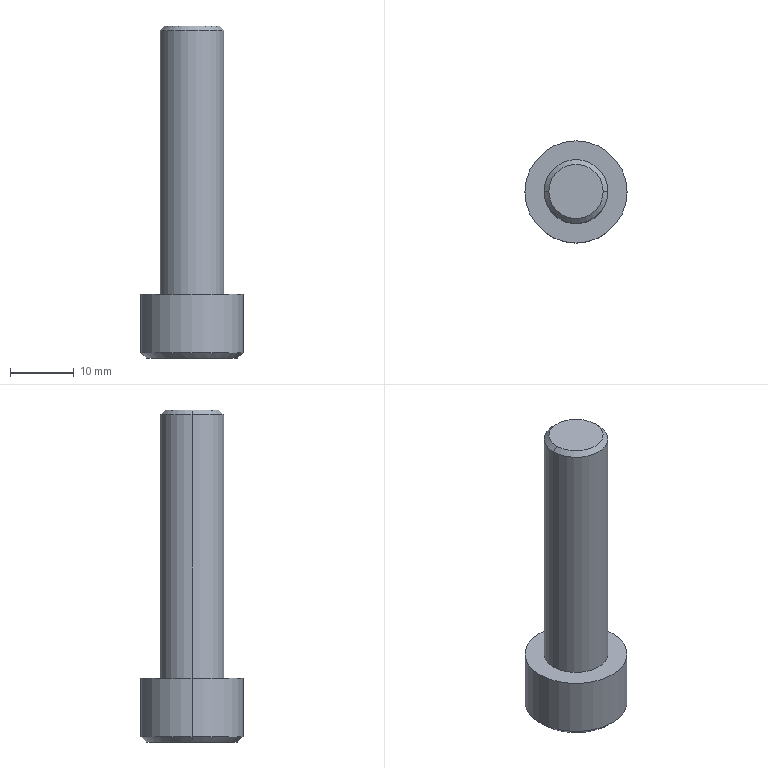Part | Creo | 1 solid | 18 faces | box 16 x 16 x 52 mm | volume 4953 mm3 | plane 10 | cylinder 4 | cone 4 | commonest cylinder face diameters 10 x2 16 x2
STEP:
#1=CARTESIAN_POINT('',(-184.,-161.,61.5));
#2=VERTEX_POINT('',#1);
#3=CARTESIAN_POINT('',(-200.,-161.,61.5));
#4=VERTEX_POINT('',#3);
#5=CARTESIAN_POINT('',(-192.,-161.,61.5));
#6=DIRECTION('',(0.,0.,1.));
#7=DIRECTION('',(1.,0.,0.));
#8=AXIS2_PLACEMENT_3D('',#5,#6,#7);
#9=CIRCLE('',#8,8.);
#10=EDGE_CURVE('',#2,#4,#9,.T.);
#11=ORIENTED_EDGE('',*,*,#10,.F.);
#12=CARTESIAN_POINT('',(-192.,-161.,61.5));
#13=DIRECTION('',(0.,0.,1.));
#14=DIRECTION('',(-1.,0.,0.));
#15=AXIS2_PLACEMENT_3D('',#12,#13,#14);
#16=CIRCLE('',#15,8.);
#17=EDGE_CURVE('',#4,#2,#16,.T.);
#18=ORIENTED_EDGE('',*,*,#17,.F.);
#19=EDGE_LOOP('',(#11,#18));
#20=FACE_OUTER_BOUND('',#19,.F.);
#21=CARTESIAN_POINT('',(-197.,-161.,61.5));
#22=VERTEX_POINT('',#21);
#23=CARTESIAN_POINT('',(-187.,-161.,61.5));
#24=VERTEX_POINT('',#23);
#25=CARTESIAN_POINT('',(-192.,-161.,61.5));
#26=DIRECTION('',(0.,0.,-1.));
#27=DIRECTION('',(-1.,0.,0.));
#28=AXIS2_PLACEMENT_3D('',#25,#26,#27);
#29=CIRCLE('',#28,5.);
#30=EDGE_CURVE('',#22,#24,#29,.T.);
#31=ORIENTED_EDGE('',*,*,#30,.F.);
#32=CARTESIAN_POINT('',(-192.,-161.,61.5));
#33=DIRECTION('',(0.,0.,-1.));
#34=DIRECTION('',(1.,0.,0.));
#35=AXIS2_PLACEMENT_3D('',#32,#33,#34);
#36=CIRCLE('',#35,5.);
#37=EDGE_CURVE('',#24,#22,#36,.T.);
#38=ORIENTED_EDGE('',*,*,#37,.F.);
#39=EDGE_LOOP('',(#31,#38));
#40=FACE_BOUND('',#39,.F.);
#41=CARTESIAN_POINT('',(-192.,-161.,61.5));
#42=DIRECTION('',(0.,0.,1.));
#43=DIRECTION('',(-1.,0.,0.));
#44=AXIS2_PLACEMENT_3D('',#41,#42,#43);
#45=PLANE('',#44);
#46=ADVANCED_FACE('',(#20,#40),#45,.T.);
#47=CARTESIAN_POINT('',(-187.,-161.,102.75));
#48=VERTEX_POINT('',#47);
#49=CARTESIAN_POINT('',(-197.,-161.,102.75));
#50=VERTEX_POINT('',#49);
#51=CARTESIAN_POINT('',(-192.,-161.,102.75));
#52=DIRECTION('',(0.,0.,1.));
#53=DIRECTION('',(1.,0.,0.));
#54=AXIS2_PLACEMENT_3D('',#51,#52,#53);
#55=CIRCLE('',#54,5.);
#56=EDGE_CURVE('',#48,#50,#55,.T.);
#57=ORIENTED_EDGE('',*,*,#56,.T.);
#58=CARTESIAN_POINT('',(-197.,-161.,61.5));
#59=DIRECTION('',(0.,0.,1.));
#60=VECTOR('',#59,41.25);
#61=LINE('',#58,#60);
#62=EDGE_CURVE('',#22,#50,#61,.T.);
#63=ORIENTED_EDGE('',*,*,#62,.F.);
#64=ORIENTED_EDGE('',*,*,#30,.T.);
#65=CARTESIAN_POINT('',(-187.,-161.,61.5));
#66=DIRECTION('',(0.,0.,1.));
#67=VECTOR('',#66,41.25);
#68=LINE('',#65,#67);
#69=EDGE_CURVE('',#24,#48,#68,.T.);
#70=ORIENTED_EDGE('',*,*,#69,.T.);
#71=EDGE_LOOP('',(#57,#63,#64,#70));
#72=FACE_OUTER_BOUND('',#71,.F.);
#73=CARTESIAN_POINT('',(-192.,-161.,21.5));
#74=DIRECTION('',(0.,0.,1.));
#75=DIRECTION('',(-1.,0.,0.));
#76=AXIS2_PLACEMENT_3D('',#73,#74,#75);
#77=CYLINDRICAL_SURFACE('',#76,5.);
#78=ADVANCED_FACE('',(#72),#77,.T.);
#79=CARTESIAN_POINT('',(-187.75,-161.,103.5));
#80=VERTEX_POINT('',#79);
#81=CARTESIAN_POINT('',(-196.25,-161.,103.5));
#82=VERTEX_POINT('',#81);
#83=CARTESIAN_POINT('',(-192.,-161.,103.5));
#84=DIRECTION('',(0.,0.,1.));
#85=DIRECTION('',(1.,0.,0.));
#86=AXIS2_PLACEMENT_3D('',#83,#84,#85);
#87=CIRCLE('',#86,4.25);
#88=EDGE_CURVE('',#80,#82,#87,.T.);
#89=ORIENTED_EDGE('',*,*,#88,.T.);
#90=CARTESIAN_POINT('',(-196.25,-161.,103.5));
#91=DIRECTION('',(-0.7071,0.,-0.7071));
#92=VECTOR('',#91,1.061);
#93=LINE('',#90,#92);
#94=EDGE_CURVE('',#82,#50,#93,.T.);
#95=ORIENTED_EDGE('',*,*,#94,.T.);
#96=ORIENTED_EDGE('',*,*,#56,.F.);
#97=CARTESIAN_POINT('',(-187.75,-161.,103.5));
#98=DIRECTION('',(0.7071,0.,-0.7071));
#99=VECTOR('',#98,1.061);
#100=LINE('',#97,#99);
#101=EDGE_CURVE('',#80,#48,#100,.T.);
#102=ORIENTED_EDGE('',*,*,#101,.F.);
#103=EDGE_LOOP('',(#89,#95,#96,#102));
#104=FACE_OUTER_BOUND('',#103,.F.);
#105=CARTESIAN_POINT('',(-192.,-161.,103.125));
#106=DIRECTION('',(0.,0.,-1.));
#107=DIRECTION('',(1.,0.,0.));
#108=AXIS2_PLACEMENT_3D('',#105,#106,#107);
#109=CONICAL_SURFACE('',#108,4.625,45.);
#110=ADVANCED_FACE('',(#104),#109,.T.);
#111=CARTESIAN_POINT('',(-192.,-161.,103.5));
#112=DIRECTION('',(0.,0.,1.));
#113=DIRECTION('',(-1.,0.,0.));
#114=AXIS2_PLACEMENT_3D('',#111,#112,#113);
#115=CIRCLE('',#114,4.25);
#116=EDGE_CURVE('',#82,#80,#115,.T.);
#117=ORIENTED_EDGE('',*,*,#116,.F.);
#118=ORIENTED_EDGE('',*,*,#88,.F.);
#119=EDGE_LOOP('',(#117,#118));
#120=FACE_OUTER_BOUND('',#119,.F.);
#121=CARTESIAN_POINT('',(-192.,-161.,103.5));
#122=DIRECTION('',(0.,0.,1.));
#123=DIRECTION('',(-1.,0.,0.));
#124=AXIS2_PLACEMENT_3D('',#121,#122,#123);
#125=PLANE('',#124);
#126=ADVANCED_FACE('',(#120),#125,.T.);
#127=ORIENTED_EDGE('',*,*,#116,.T.);
#128=ORIENTED_EDGE('',*,*,#101,.T.);
#129=CARTESIAN_POINT('',(-192.,-161.,102.75));
#130=DIRECTION('',(0.,0.,1.));
#131=DIRECTION('',(-1.,0.,0.));
#132=AXIS2_PLACEMENT_3D('',#129,#130,#131);
#133=CIRCLE('',#132,5.);
#134=EDGE_CURVE('',#50,#48,#133,.T.);
#135=ORIENTED_EDGE('',*,*,#134,.F.);
#136=ORIENTED_EDGE('',*,*,#94,.F.);
#137=EDGE_LOOP('',(#127,#128,#135,#136));
#138=FACE_OUTER_BOUND('',#137,.F.);
#139=CARTESIAN_POINT('',(-192.,-161.,103.125));
#140=DIRECTION('',(0.,0.,-1.));
#141=DIRECTION('',(1.,0.,0.));
#142=AXIS2_PLACEMENT_3D('',#139,#140,#141);
#143=CONICAL_SURFACE('',#142,4.625,45.);
#144=ADVANCED_FACE('',(#138),#143,.T.);
#145=ORIENTED_EDGE('',*,*,#134,.T.);
#146=ORIENTED_EDGE('',*,*,#69,.F.);
#147=ORIENTED_EDGE('',*,*,#37,.T.);
#148=ORIENTED_EDGE('',*,*,#62,.T.);
#149=EDGE_LOOP('',(#145,#146,#147,#148));
#150=FACE_OUTER_BOUND('',#149,.F.);
#151=CARTESIAN_POINT('',(-192.,-161.,21.5));
#152=DIRECTION('',(0.,0.,1.));
#153=DIRECTION('',(-1.,0.,0.));
#154=AXIS2_PLACEMENT_3D('',#151,#152,#153);
#155=CYLINDRICAL_SURFACE('',#154,5.);
#156=ADVANCED_FACE('',(#150),#155,.T.);
#157=CARTESIAN_POINT('',(-200.,-161.,52.3));
#158=VERTEX_POINT('',#157);
#159=CARTESIAN_POINT('',(-184.,-161.,52.3));
#160=VERTEX_POINT('',#159);
#161=CARTESIAN_POINT('',(-192.,-161.,52.3));
#162=DIRECTION('',(0.,0.,-1.));
#163=DIRECTION('',(-1.,0.,0.));
#164=AXIS2_PLACEMENT_3D('',#161,#162,#163);
#165=CIRCLE('',#164,8.);
#166=EDGE_CURVE('',#158,#160,#165,.T.);
#167=ORIENTED_EDGE('',*,*,#166,.T.);
#168=CARTESIAN_POINT('',(-184.,-161.,52.3));
#169=DIRECTION('',(0.,0.,1.));
#170=VECTOR('',#169,9.2);
#171=LINE('',#168,#170);
#172=EDGE_CURVE('',#160,#2,#171,.T.);
#173=ORIENTED_EDGE('',*,*,#172,.T.);
#174=ORIENTED_EDGE('',*,*,#10,.T.);
#175=CARTESIAN_POINT('',(-200.,-161.,52.3));
#176=DIRECTION('',(0.,0.,1.));
#177=VECTOR('',#176,9.2);
#178=LINE('',#175,#177);
#179=EDGE_CURVE('',#158,#4,#178,.T.);
#180=ORIENTED_EDGE('',*,*,#179,.F.);
#181=EDGE_LOOP('',(#167,#173,#174,#180));
#182=FACE_OUTER_BOUND('',#181,.F.);
#183=CARTESIAN_POINT('',(-192.,-161.,49.5));
#184=DIRECTION('',(0.,0.,1.));
#185=DIRECTION('',(-1.,0.,0.));
#186=AXIS2_PLACEMENT_3D('',#183,#184,#185);
#187=CYLINDRICAL_SURFACE('',#186,8.);
#188=ADVANCED_FACE('',(#182),#187,.T.);
#189=CARTESIAN_POINT('',(-199.2,-161.,51.5));
#190=VERTEX_POINT('',#189);
#191=CARTESIAN_POINT('',(-184.8,-161.,51.5));
#192=VERTEX_POINT('',#191);
#193=CARTESIAN_POINT('',(-192.,-161.,51.5));
#194=DIRECTION('',(0.,0.,-1.));
#195=DIRECTION('',(-1.,0.,0.));
#196=AXIS2_PLACEMENT_3D('',#193,#194,#195);
#197=CIRCLE('',#196,7.2);
#198=EDGE_CURVE('',#190,#192,#197,.T.);
#199=ORIENTED_EDGE('',*,*,#198,.T.);
#200=CARTESIAN_POINT('',(-184.8,-161.,51.5));
#201=DIRECTION('',(0.7071,0.,0.7071));
#202=VECTOR('',#201,1.131);
#203=LINE('',#200,#202);
#204=EDGE_CURVE('',#192,#160,#203,.T.);
#205=ORIENTED_EDGE('',*,*,#204,.T.);
#206=ORIENTED_EDGE('',*,*,#166,.F.);
#207=CARTESIAN_POINT('',(-199.2,-161.,51.5));
#208=DIRECTION('',(-0.7071,0.,0.7071));
#209=VECTOR('',#208,1.131);
#210=LINE('',#207,#209);
#211=EDGE_CURVE('',#190,#158,#210,.T.);
#212=ORIENTED_EDGE('',*,*,#211,.F.);
#213=EDGE_LOOP('',(#199,#205,#206,#212));
#214=FACE_OUTER_BOUND('',#213,.F.);
#215=CARTESIAN_POINT('',(-192.,-161.,51.9));
#216=DIRECTION('',(0.,0.,1.));
#217=DIRECTION('',(-1.,0.,0.));
#218=AXIS2_PLACEMENT_3D('',#215,#216,#217);
#219=CONICAL_SURFACE('',#218,7.6,45.);
#220=ADVANCED_FACE('',(#214),#219,.T.);
#221=ORIENTED_EDGE('',*,*,#198,.F.);
#222=CARTESIAN_POINT('',(-192.,-161.,51.5));
#223=DIRECTION('',(0.,0.,-1.));
#224=DIRECTION('',(1.,0.,0.));
#225=AXIS2_PLACEMENT_3D('',#222,#223,#224);
#226=CIRCLE('',#225,7.2);
#227=EDGE_CURVE('',#192,#190,#226,.T.);
#228=ORIENTED_EDGE('',*,*,#227,.F.);
#229=EDGE_LOOP('',(#221,#228));
#230=FACE_OUTER_BOUND('',#229,.F.);
#231=CARTESIAN_POINT('',(-192.,-165.619,51.5));
#232=VERTEX_POINT('',#231);
#233=CARTESIAN_POINT('',(-188.,-163.309,51.5));
#234=VERTEX_POINT('',#233);
#235=CARTESIAN_POINT('',(-192.,-165.619,51.5));
#236=DIRECTION('',(0.866,0.5,0.));
#237=VECTOR('',#236,4.619);
#238=LINE('',#235,#237);
#239=EDGE_CURVE('',#232,#234,#238,.T.);
#240=ORIENTED_EDGE('',*,*,#239,.F.);
#241=CARTESIAN_POINT('',(-196.,-163.309,51.5));
#242=VERTEX_POINT('',#241);
#243=CARTESIAN_POINT('',(-196.,-163.309,51.5));
#244=DIRECTION('',(0.866,-0.5,0.));
#245=VECTOR('',#244,4.619);
#246=LINE('',#243,#245);
#247=EDGE_CURVE('',#242,#232,#246,.T.);
#248=ORIENTED_EDGE('',*,*,#247,.F.);
#249=CARTESIAN_POINT('',(-196.,-158.691,51.5));
#250=VERTEX_POINT('',#249);
#251=CARTESIAN_POINT('',(-196.,-163.309,51.5));
#252=DIRECTION('',(0.,1.,0.));
#253=VECTOR('',#252,4.619);
#254=LINE('',#251,#253);
#255=EDGE_CURVE('',#242,#250,#254,.T.);
#256=ORIENTED_EDGE('',*,*,#255,.T.);
#257=CARTESIAN_POINT('',(-192.,-156.381,51.5));
#258=VERTEX_POINT('',#257);
#259=CARTESIAN_POINT('',(-192.,-156.381,51.5));
#260=DIRECTION('',(-0.866,-0.5,0.));
#261=VECTOR('',#260,4.619);
#262=LINE('',#259,#261);
#263=EDGE_CURVE('',#258,#250,#262,.T.);
#264=ORIENTED_EDGE('',*,*,#263,.F.);
#265=CARTESIAN_POINT('',(-188.,-158.691,51.5));
#266=VERTEX_POINT('',#265);
#267=CARTESIAN_POINT('',(-188.,-158.691,51.5));
#268=DIRECTION('',(-0.866,0.5,0.));
#269=VECTOR('',#268,4.619);
#270=LINE('',#267,#269);
#271=EDGE_CURVE('',#266,#258,#270,.T.);
#272=ORIENTED_EDGE('',*,*,#271,.F.);
#273=CARTESIAN_POINT('',(-188.,-158.691,51.5));
#274=DIRECTION('',(0.,-1.,0.));
#275=VECTOR('',#274,4.619);
#276=LINE('',#273,#275);
#277=EDGE_CURVE('',#266,#234,#276,.T.);
#278=ORIENTED_EDGE('',*,*,#277,.T.);
#279=EDGE_LOOP('',(#240,#248,#256,#264,#272,#278));
#280=FACE_BOUND('',#279,.F.);
#281=CARTESIAN_POINT('',(-192.,-161.,51.5));
#282=DIRECTION('',(0.,0.,1.));
#283=DIRECTION('',(-1.,0.,0.));
#284=AXIS2_PLACEMENT_3D('',#281,#282,#283);
#285=PLANE('',#284);
#286=ADVANCED_FACE('',(#230,#280),#285,.F.);
#287=ORIENTED_EDGE('',*,*,#227,.T.);
#288=ORIENTED_EDGE('',*,*,#211,.T.);
#289=CARTESIAN_POINT('',(-192.,-161.,52.3));
#290=DIRECTION('',(0.,0.,-1.));
#291=DIRECTION('',(1.,0.,0.));
#292=AXIS2_PLACEMENT_3D('',#289,#290,#291);
#293=CIRCLE('',#292,8.);
#294=EDGE_CURVE('',#160,#158,#293,.T.);
#295=ORIENTED_EDGE('',*,*,#294,.F.);
#296=ORIENTED_EDGE('',*,*,#204,.F.);
#297=EDGE_LOOP('',(#287,#288,#295,#296));
#298=FACE_OUTER_BOUND('',#297,.F.);
#299=CARTESIAN_POINT('',(-192.,-161.,51.9));
#300=DIRECTION('',(0.,0.,1.));
#301=DIRECTION('',(-1.,0.,0.));
#302=AXIS2_PLACEMENT_3D('',#299,#300,#301);
#303=CONICAL_SURFACE('',#302,7.6,45.);
#304=ADVANCED_FACE('',(#298),#303,.T.);
#305=ORIENTED_EDGE('',*,*,#294,.T.);
#306=ORIENTED_EDGE('',*,*,#179,.T.);
#307=ORIENTED_EDGE('',*,*,#17,.T.);
#308=ORIENTED_EDGE('',*,*,#172,.F.);
#309=EDGE_LOOP('',(#305,#306,#307,#308));
#310=FACE_OUTER_BOUND('',#309,.F.);
#311=CARTESIAN_POINT('',(-192.,-161.,49.5));
#312=DIRECTION('',(0.,0.,1.));
#313=DIRECTION('',(-1.,0.,0.));
#314=AXIS2_PLACEMENT_3D('',#311,#312,#313);
#315=CYLINDRICAL_SURFACE('',#314,8.);
#316=ADVANCED_FACE('',(#310),#315,.T.);
#317=ORIENTED_EDGE('',*,*,#239,.T.);
#318=CARTESIAN_POINT('',(-188.,-163.309,57.5));
#319=VERTEX_POINT('',#318);
#320=CARTESIAN_POINT('',(-188.,-163.309,51.5));
#321=DIRECTION('',(0.,0.,1.));
#322=VECTOR('',#321,6.);
#323=LINE('',#320,#322);
#324=EDGE_CURVE('',#234,#319,#323,.T.);
#325=ORIENTED_EDGE('',*,*,#324,.T.);
#326=CARTESIAN_POINT('',(-192.,-165.619,57.5));
#327=VERTEX_POINT('',#326);
#328=CARTESIAN_POINT('',(-188.,-163.309,57.5));
#329=DIRECTION('',(-0.866,-0.5,0.));
#330=VECTOR('',#329,4.619);
#331=LINE('',#328,#330);
#332=EDGE_CURVE('',#319,#327,#331,.T.);
#333=ORIENTED_EDGE('',*,*,#332,.T.);
#334=CARTESIAN_POINT('',(-192.,-165.619,51.5));
#335=DIRECTION('',(0.,0.,1.));
#336=VECTOR('',#335,6.);
#337=LINE('',#334,#336);
#338=EDGE_CURVE('',#232,#327,#337,.T.);
#339=ORIENTED_EDGE('',*,*,#338,.F.);
#340=EDGE_LOOP('',(#317,#325,#333,#339));
#341=FACE_OUTER_BOUND('',#340,.F.);
#342=CARTESIAN_POINT('',(-192.,-165.619,57.5));
#343=DIRECTION('',(0.5,-0.866,0.));
#344=DIRECTION('',(0.866,0.5,0.));
#345=AXIS2_PLACEMENT_3D('',#342,#343,#344);
#346=PLANE('',#345);
#347=ADVANCED_FACE('',(#341),#346,.F.);
#348=ORIENTED_EDGE('',*,*,#277,.F.);
#349=CARTESIAN_POINT('',(-188.,-158.691,57.5));
#350=VERTEX_POINT('',#349);
#351=CARTESIAN_POINT('',(-188.,-158.691,51.5));
#352=DIRECTION('',(0.,0.,1.));
#353=VECTOR('',#352,6.);
#354=LINE('',#351,#353);
#355=EDGE_CURVE('',#266,#350,#354,.T.);
#356=ORIENTED_EDGE('',*,*,#355,.T.);
#357=CARTESIAN_POINT('',(-188.,-158.691,57.5));
#358=DIRECTION('',(0.,-1.,0.));
#359=VECTOR('',#358,4.619);
#360=LINE('',#357,#359);
#361=EDGE_CURVE('',#350,#319,#360,.T.);
#362=ORIENTED_EDGE('',*,*,#361,.T.);
#363=ORIENTED_EDGE('',*,*,#324,.F.);
#364=EDGE_LOOP('',(#348,#356,#362,#363));
#365=FACE_OUTER_BOUND('',#364,.F.);
#366=CARTESIAN_POINT('',(-188.,-163.309,57.5));
#367=DIRECTION('',(1.,0.,0.));
#368=DIRECTION('',(0.,0.,1.));
#369=AXIS2_PLACEMENT_3D('',#366,#367,#368);
#370=PLANE('',#369);
#371=ADVANCED_FACE('',(#365),#370,.F.);
#372=ORIENTED_EDGE('',*,*,#271,.T.);
#373=CARTESIAN_POINT('',(-192.,-156.381,57.5));
#374=VERTEX_POINT('',#373);
#375=CARTESIAN_POINT('',(-192.,-156.381,51.5));
#376=DIRECTION('',(0.,0.,1.));
#377=VECTOR('',#376,6.);
#378=LINE('',#375,#377);
#379=EDGE_CURVE('',#258,#374,#378,.T.);
#380=ORIENTED_EDGE('',*,*,#379,.T.);
#381=CARTESIAN_POINT('',(-192.,-156.381,57.5));
#382=DIRECTION('',(0.866,-0.5,0.));
#383=VECTOR('',#382,4.619);
#384=LINE('',#381,#383);
#385=EDGE_CURVE('',#374,#350,#384,.T.);
#386=ORIENTED_EDGE('',*,*,#385,.T.);
#387=ORIENTED_EDGE('',*,*,#355,.F.);
#388=EDGE_LOOP('',(#372,#380,#386,#387));
#389=FACE_OUTER_BOUND('',#388,.F.);
#390=CARTESIAN_POINT('',(-188.,-158.691,57.5));
#391=DIRECTION('',(0.5,0.866,0.));
#392=DIRECTION('',(-0.866,0.5,0.));
#393=AXIS2_PLACEMENT_3D('',#390,#391,#392);
#394=PLANE('',#393);
#395=ADVANCED_FACE('',(#389),#394,.F.);
#396=ORIENTED_EDGE('',*,*,#263,.T.);
#397=CARTESIAN_POINT('',(-196.,-158.691,57.5));
#398=VERTEX_POINT('',#397);
#399=CARTESIAN_POINT('',(-196.,-158.691,51.5));
#400=DIRECTION('',(0.,0.,1.));
#401=VECTOR('',#400,6.);
#402=LINE('',#399,#401);
#403=EDGE_CURVE('',#250,#398,#402,.T.);
#404=ORIENTED_EDGE('',*,*,#403,.T.);
#405=CARTESIAN_POINT('',(-196.,-158.691,57.5));
#406=DIRECTION('',(0.866,0.5,0.));
#407=VECTOR('',#406,4.619);
#408=LINE('',#405,#407);
#409=EDGE_CURVE('',#398,#374,#408,.T.);
#410=ORIENTED_EDGE('',*,*,#409,.T.);
#411=ORIENTED_EDGE('',*,*,#379,.F.);
#412=EDGE_LOOP('',(#396,#404,#410,#411));
#413=FACE_OUTER_BOUND('',#412,.F.);
#414=CARTESIAN_POINT('',(-192.,-156.381,57.5));
#415=DIRECTION('',(-0.5,0.866,0.));
#416=DIRECTION('',(-0.866,-0.5,0.));
#417=AXIS2_PLACEMENT_3D('',#414,#415,#416);
#418=PLANE('',#417);
#419=ADVANCED_FACE('',(#413),#418,.F.);
#420=ORIENTED_EDGE('',*,*,#255,.F.);
#421=CARTESIAN_POINT('',(-196.,-163.309,57.5));
#422=VERTEX_POINT('',#421);
#423=CARTESIAN_POINT('',(-196.,-163.309,51.5));
#424=DIRECTION('',(0.,0.,1.));
#425=VECTOR('',#424,6.);
#426=LINE('',#423,#425);
#427=EDGE_CURVE('',#242,#422,#426,.T.);
#428=ORIENTED_EDGE('',*,*,#427,.T.);
#429=CARTESIAN_POINT('',(-196.,-163.309,57.5));
#430=DIRECTION('',(0.,1.,0.));
#431=VECTOR('',#430,4.619);
#432=LINE('',#429,#431);
#433=EDGE_CURVE('',#422,#398,#432,.T.);
#434=ORIENTED_EDGE('',*,*,#433,.T.);
#435=ORIENTED_EDGE('',*,*,#403,.F.);
#436=EDGE_LOOP('',(#420,#428,#434,#435));
#437=FACE_OUTER_BOUND('',#436,.F.);
#438=CARTESIAN_POINT('',(-196.,-158.691,57.5));
#439=DIRECTION('',(-1.,0.,0.));
#440=DIRECTION('',(0.,0.,-1.));
#441=AXIS2_PLACEMENT_3D('',#438,#439,#440);
#442=PLANE('',#441);
#443=ADVANCED_FACE('',(#437),#442,.F.);
#444=ORIENTED_EDGE('',*,*,#247,.T.);
#445=ORIENTED_EDGE('',*,*,#338,.T.);
#446=CARTESIAN_POINT('',(-192.,-165.619,57.5));
#447=DIRECTION('',(-0.866,0.5,0.));
#448=VECTOR('',#447,4.619);
#449=LINE('',#446,#448);
#450=EDGE_CURVE('',#327,#422,#449,.T.);
#451=ORIENTED_EDGE('',*,*,#450,.T.);
#452=ORIENTED_EDGE('',*,*,#427,.F.);
#453=EDGE_LOOP('',(#444,#445,#451,#452));
#454=FACE_OUTER_BOUND('',#453,.F.);
#455=CARTESIAN_POINT('',(-196.,-163.309,57.5));
#456=DIRECTION('',(-0.5,-0.866,0.));
#457=DIRECTION('',(0.866,-0.5,0.));
#458=AXIS2_PLACEMENT_3D('',#455,#456,#457);
#459=PLANE('',#458);
#460=ADVANCED_FACE('',(#454),#459,.F.);
#461=ORIENTED_EDGE('',*,*,#450,.F.);
#462=ORIENTED_EDGE('',*,*,#332,.F.);
#463=ORIENTED_EDGE('',*,*,#361,.F.);
#464=ORIENTED_EDGE('',*,*,#385,.F.);
#465=ORIENTED_EDGE('',*,*,#409,.F.);
#466=ORIENTED_EDGE('',*,*,#433,.F.);
#467=EDGE_LOOP('',(#461,#462,#463,#464,#465,#466));
#468=FACE_OUTER_BOUND('',#467,.F.);
#469=CARTESIAN_POINT('',(-188.,-167.928,57.5));
#470=DIRECTION('',(0.,0.,-1.));
#471=DIRECTION('',(1.,0.,0.));
#472=AXIS2_PLACEMENT_3D('',#469,#470,#471);
#473=PLANE('',#472);
#474=ADVANCED_FACE('',(#468),#473,.T.);
#475=CLOSED_SHELL('',(#46,#78,#110,#126,#144,#156,#188,#220,#286,#304,#316,#347,#371,#395,#419,#443,#460,#474));
#476=MANIFOLD_SOLID_BREP('',#475);
#477=(LENGTH_UNIT()NAMED_UNIT(*)SI_UNIT(.MILLI.,.METRE.));
#478=UNCERTAINTY_MEASURE_WITH_UNIT(LENGTH_MEASURE(0.005671),#477,'','');
#479=(NAMED_UNIT(*)PLANE_ANGLE_UNIT()SI_UNIT($,.RADIAN.));
#480=PLANE_ANGLE_MEASURE_WITH_UNIT(PLANE_ANGLE_MEASURE(0.01745),#479);
#481=(CONVERSION_BASED_UNIT('DEGREE',#480)NAMED_UNIT(*)PLANE_ANGLE_UNIT());
#482=(NAMED_UNIT(*)SI_UNIT($,.STERADIAN.)SOLID_ANGLE_UNIT());
#483=(GEOMETRIC_REPRESENTATION_CONTEXT(3)GLOBAL_UNCERTAINTY_ASSIGNED_CONTEXT((#478))GLOBAL_UNIT_ASSIGNED_CONTEXT((#477,#481,#482))REPRESENTATION_CONTEXT('',''));
#484=ADVANCED_BREP_SHAPE_REPRESENTATION('',(#476),#483);